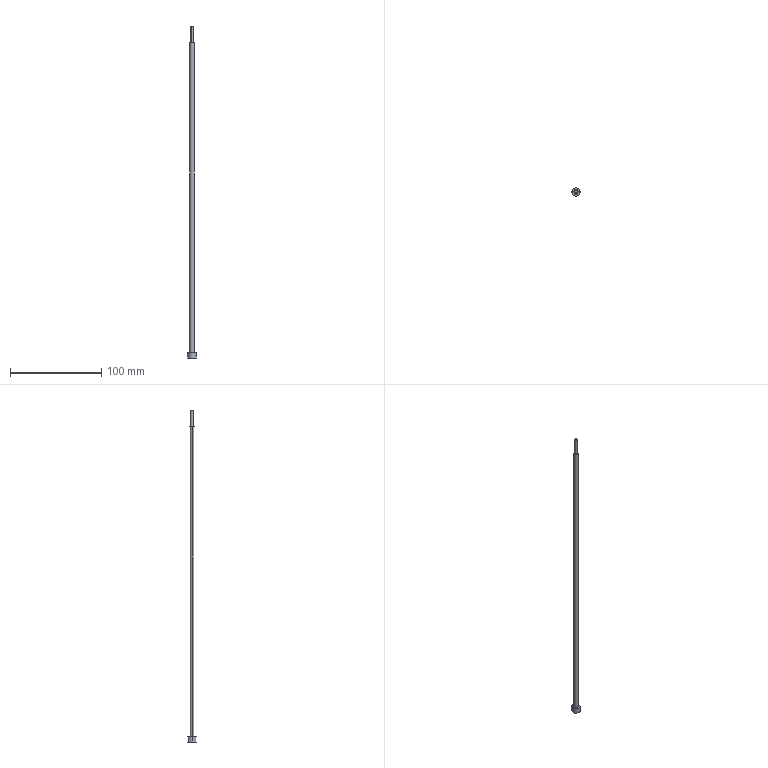Part | Creo | 1 solid | 12 faces | box 9 x 9 x 363.491 mm | volume 5926 mm3 | cylinder 6 | plane 4 | cone 2 | commonest cylinder face diameters 3.214 x2 4.5 x2 9 x2
STEP:
#1=CARTESIAN_POINT('',(-76.601,-142.631,-319.5));
#2=VERTEX_POINT('',#1);
#3=CARTESIAN_POINT('',(-72.101,-142.631,-319.5));
#4=VERTEX_POINT('',#3);
#5=CARTESIAN_POINT('',(-74.351,-142.631,-319.5));
#6=DIRECTION('',(0.,0.,-1.));
#7=DIRECTION('',(-1.,0.,0.));
#8=AXIS2_PLACEMENT_3D('',#5,#6,#7);
#9=CIRCLE('',#8,2.25);
#10=EDGE_CURVE('',#2,#4,#9,.T.);
#11=ORIENTED_EDGE('',*,*,#10,.T.);
#12=CARTESIAN_POINT('',(-72.101,-142.631,19.789));
#13=VERTEX_POINT('',#12);
#14=CARTESIAN_POINT('',(-72.101,-142.631,-319.5));
#15=DIRECTION('',(0.,0.,1.));
#16=VECTOR('',#15,339.289);
#17=LINE('',#14,#16);
#18=EDGE_CURVE('',#4,#13,#17,.T.);
#19=ORIENTED_EDGE('',*,*,#18,.T.);
#20=CARTESIAN_POINT('',(-76.601,-142.631,19.789));
#21=VERTEX_POINT('',#20);
#22=CARTESIAN_POINT('',(-74.351,-142.631,19.789));
#23=DIRECTION('',(0.,0.,1.));
#24=DIRECTION('',(1.,0.,0.));
#25=AXIS2_PLACEMENT_3D('',#22,#23,#24);
#26=CIRCLE('',#25,2.25);
#27=EDGE_CURVE('',#13,#21,#26,.T.);
#28=ORIENTED_EDGE('',*,*,#27,.T.);
#29=CARTESIAN_POINT('',(-76.601,-142.631,-319.5));
#30=DIRECTION('',(0.,0.,1.));
#31=VECTOR('',#30,339.289);
#32=LINE('',#29,#31);
#33=EDGE_CURVE('',#2,#21,#32,.T.);
#34=ORIENTED_EDGE('',*,*,#33,.F.);
#35=EDGE_LOOP('',(#11,#19,#28,#34));
#36=FACE_OUTER_BOUND('',#35,.F.);
#37=CARTESIAN_POINT('',(-74.351,-142.631,-310.5));
#38=DIRECTION('',(0.,0.,1.));
#39=DIRECTION('',(1.,0.,0.));
#40=AXIS2_PLACEMENT_3D('',#37,#38,#39);
#41=CYLINDRICAL_SURFACE('',#40,2.25);
#42=ADVANCED_FACE('',(#36),#41,.T.);
#43=CARTESIAN_POINT('',(-78.851,-142.631,-319.5));
#44=VERTEX_POINT('',#43);
#45=CARTESIAN_POINT('',(-69.851,-142.631,-319.5));
#46=VERTEX_POINT('',#45);
#47=CARTESIAN_POINT('',(-74.351,-142.631,-319.5));
#48=DIRECTION('',(0.,0.,1.));
#49=DIRECTION('',(-1.,0.,0.));
#50=AXIS2_PLACEMENT_3D('',#47,#48,#49);
#51=CIRCLE('',#50,4.5);
#52=EDGE_CURVE('',#44,#46,#51,.T.);
#53=ORIENTED_EDGE('',*,*,#52,.F.);
#54=CARTESIAN_POINT('',(-74.351,-142.631,-319.5));
#55=DIRECTION('',(0.,0.,1.));
#56=DIRECTION('',(1.,0.,0.));
#57=AXIS2_PLACEMENT_3D('',#54,#55,#56);
#58=CIRCLE('',#57,4.5);
#59=EDGE_CURVE('',#46,#44,#58,.T.);
#60=ORIENTED_EDGE('',*,*,#59,.F.);
#61=EDGE_LOOP('',(#53,#60));
#62=FACE_OUTER_BOUND('',#61,.F.);
#63=CARTESIAN_POINT('',(-74.351,-142.631,-319.5));
#64=DIRECTION('',(0.,0.,-1.));
#65=DIRECTION('',(1.,0.,0.));
#66=AXIS2_PLACEMENT_3D('',#63,#64,#65);
#67=CIRCLE('',#66,2.25);
#68=EDGE_CURVE('',#4,#2,#67,.T.);
#69=ORIENTED_EDGE('',*,*,#68,.F.);
#70=ORIENTED_EDGE('',*,*,#10,.F.);
#71=EDGE_LOOP('',(#69,#70));
#72=FACE_BOUND('',#71,.F.);
#73=CARTESIAN_POINT('',(-74.351,-142.631,-319.5));
#74=DIRECTION('',(0.,0.,1.));
#75=DIRECTION('',(1.,0.,0.));
#76=AXIS2_PLACEMENT_3D('',#73,#74,#75);
#77=PLANE('',#76);
#78=ADVANCED_FACE('',(#62,#72),#77,.T.);
#79=ORIENTED_EDGE('',*,*,#68,.T.);
#80=ORIENTED_EDGE('',*,*,#33,.T.);
#81=CARTESIAN_POINT('',(-74.351,-142.631,19.789));
#82=DIRECTION('',(0.,0.,1.));
#83=DIRECTION('',(-1.,0.,0.));
#84=AXIS2_PLACEMENT_3D('',#81,#82,#83);
#85=CIRCLE('',#84,2.25);
#86=EDGE_CURVE('',#21,#13,#85,.T.);
#87=ORIENTED_EDGE('',*,*,#86,.T.);
#88=ORIENTED_EDGE('',*,*,#18,.F.);
#89=EDGE_LOOP('',(#79,#80,#87,#88));
#90=FACE_OUTER_BOUND('',#89,.F.);
#91=CARTESIAN_POINT('',(-74.351,-142.631,-310.5));
#92=DIRECTION('',(0.,0.,1.));
#93=DIRECTION('',(1.,0.,0.));
#94=AXIS2_PLACEMENT_3D('',#91,#92,#93);
#95=CYLINDRICAL_SURFACE('',#94,2.25);
#96=ADVANCED_FACE('',(#90),#95,.T.);
#97=ORIENTED_EDGE('',*,*,#86,.F.);
#98=ORIENTED_EDGE('',*,*,#27,.F.);
#99=EDGE_LOOP('',(#97,#98));
#100=FACE_OUTER_BOUND('',#99,.F.);
#101=CARTESIAN_POINT('',(-74.351,-140.522,19.789));
#102=VERTEX_POINT('',#101);
#103=CARTESIAN_POINT('',(-72.242,-142.631,19.789));
#104=VERTEX_POINT('',#103);
#105=CARTESIAN_POINT('',(-74.351,-142.631,19.789));
#106=DIRECTION('',(0.,0.,-1.));
#107=DIRECTION('',(0.,1.,0.));
#108=AXIS2_PLACEMENT_3D('',#105,#106,#107);
#109=CIRCLE('',#108,2.109);
#110=EDGE_CURVE('',#102,#104,#109,.T.);
#111=ORIENTED_EDGE('',*,*,#110,.F.);
#112=CARTESIAN_POINT('',(-76.461,-142.631,19.789));
#113=VERTEX_POINT('',#112);
#114=CARTESIAN_POINT('',(-74.351,-142.631,19.789));
#115=DIRECTION('',(0.,0.,-1.));
#116=DIRECTION('',(-1.,0.,0.));
#117=AXIS2_PLACEMENT_3D('',#114,#115,#116);
#118=CIRCLE('',#117,2.109);
#119=EDGE_CURVE('',#113,#102,#118,.T.);
#120=ORIENTED_EDGE('',*,*,#119,.F.);
#121=CARTESIAN_POINT('',(-74.351,-142.631,19.789));
#122=DIRECTION('',(0.,0.,-1.));
#123=DIRECTION('',(1.,0.,0.));
#124=AXIS2_PLACEMENT_3D('',#121,#122,#123);
#125=CIRCLE('',#124,2.109);
#126=EDGE_CURVE('',#104,#113,#125,.T.);
#127=ORIENTED_EDGE('',*,*,#126,.F.);
#128=EDGE_LOOP('',(#111,#120,#127));
#129=FACE_BOUND('',#128,.F.);
#130=CARTESIAN_POINT('',(-0.003698,-18.777,19.789));
#131=DIRECTION('',(0.,0.,-1.));
#132=DIRECTION('',(0.,-1.,0.));
#133=AXIS2_PLACEMENT_3D('',#130,#131,#132);
#134=PLANE('',#133);
#135=ADVANCED_FACE('',(#100,#129),#134,.F.);
#136=CARTESIAN_POINT('',(-74.351,-141.024,20.291));
#137=VERTEX_POINT('',#136);
#138=CARTESIAN_POINT('',(-72.744,-142.631,20.291));
#139=VERTEX_POINT('',#138);
#140=CARTESIAN_POINT('',(-74.351,-142.631,20.291));
#141=DIRECTION('',(0.,0.,-1.));
#142=DIRECTION('',(0.,1.,0.));
#143=AXIS2_PLACEMENT_3D('',#140,#141,#142);
#144=CIRCLE('',#143,1.607);
#145=EDGE_CURVE('',#137,#139,#144,.T.);
#146=ORIENTED_EDGE('',*,*,#145,.F.);
#147=CARTESIAN_POINT('',(-75.959,-142.631,20.291));
#148=VERTEX_POINT('',#147);
#149=CARTESIAN_POINT('',(-74.351,-142.631,20.291));
#150=DIRECTION('',(0.,0.,-1.));
#151=DIRECTION('',(-1.,0.,0.));
#152=AXIS2_PLACEMENT_3D('',#149,#150,#151);
#153=CIRCLE('',#152,1.607);
#154=EDGE_CURVE('',#148,#137,#153,.T.);
#155=ORIENTED_EDGE('',*,*,#154,.F.);
#156=CARTESIAN_POINT('',(-75.959,-142.631,20.291));
#157=DIRECTION('',(-0.7071,0.,-0.7072));
#158=VECTOR('',#157,0.7099);
#159=LINE('',#156,#158);
#160=EDGE_CURVE('',#148,#113,#159,.T.);
#161=ORIENTED_EDGE('',*,*,#160,.T.);
#162=ORIENTED_EDGE('',*,*,#119,.T.);
#163=ORIENTED_EDGE('',*,*,#110,.T.);
#164=CARTESIAN_POINT('',(-72.744,-142.631,20.291));
#165=DIRECTION('',(0.7071,0.,-0.7072));
#166=VECTOR('',#165,0.7099);
#167=LINE('',#164,#166);
#168=EDGE_CURVE('',#139,#104,#167,.T.);
#169=ORIENTED_EDGE('',*,*,#168,.F.);
#170=EDGE_LOOP('',(#146,#155,#161,#162,#163,#169));
#171=FACE_OUTER_BOUND('',#170,.F.);
#172=CARTESIAN_POINT('',(-74.351,-142.631,20.04));
#173=DIRECTION('',(0.,0.,-1.));
#174=DIRECTION('',(1.,0.,0.));
#175=AXIS2_PLACEMENT_3D('',#172,#173,#174);
#176=CONICAL_SURFACE('',#175,1.858,44.996);
#177=ADVANCED_FACE('',(#171),#176,.T.);
#178=CARTESIAN_POINT('',(-74.351,-144.239,37.93));
#179=VERTEX_POINT('',#178);
#180=CARTESIAN_POINT('',(-72.744,-142.631,37.868));
#181=VERTEX_POINT('',#180);
#182=CARTESIAN_POINT('',(-74.351,-144.239,37.93));
#183=CARTESIAN_POINT('',(-74.132,-144.239,37.921));
#184=CARTESIAN_POINT('',(-73.729,-144.156,37.906));
#185=CARTESIAN_POINT('',(-73.188,-143.803,37.885));
#186=CARTESIAN_POINT('',(-72.83,-143.263,37.872));
#187=CARTESIAN_POINT('',(-72.744,-142.854,37.868));
#188=B_SPLINE_CURVE_WITH_KNOTS('',3,(#182,#183,#184,#185,#186,#187,#180),.UNSPECIFIED.,.F.,.F.,(4,1,1,1,4),(0.,0.25,0.5,0.75,1.),.UNSPECIFIED.);
#189=EDGE_CURVE('',#179,#181,#188,.T.);
#190=ORIENTED_EDGE('',*,*,#189,.T.);
#191=CARTESIAN_POINT('',(-74.351,-141.024,37.93));
#192=VERTEX_POINT('',#191);
#193=CARTESIAN_POINT('',(-72.744,-142.631,37.868));
#194=CARTESIAN_POINT('',(-72.744,-142.409,37.868));
#195=CARTESIAN_POINT('',(-72.83,-142.,37.872));
#196=CARTESIAN_POINT('',(-73.188,-141.46,37.885));
#197=CARTESIAN_POINT('',(-73.728,-141.107,37.906));
#198=CARTESIAN_POINT('',(-74.132,-141.024,37.921));
#199=CARTESIAN_POINT('',(-74.351,-141.024,37.93));
#200=B_SPLINE_CURVE_WITH_KNOTS('',3,(#193,#194,#195,#196,#197,#198,#199),.UNSPECIFIED.,.F.,.F.,(4,1,1,1,4),(0.,0.25,0.5,0.75,1.),.UNSPECIFIED.);
#201=EDGE_CURVE('',#181,#192,#200,.T.);
#202=ORIENTED_EDGE('',*,*,#201,.T.);
#203=CARTESIAN_POINT('',(-74.351,-141.024,37.93));
#204=DIRECTION('',(-0.000002985,0.000000828,-1.));
#205=VECTOR('',#204,17.639);
#206=LINE('',#203,#205);
#207=EDGE_CURVE('',#192,#137,#206,.T.);
#208=ORIENTED_EDGE('',*,*,#207,.T.);
#209=ORIENTED_EDGE('',*,*,#145,.T.);
#210=CARTESIAN_POINT('',(-74.351,-144.239,20.291));
#211=VERTEX_POINT('',#210);
#212=CARTESIAN_POINT('',(-74.351,-142.631,20.291));
#213=DIRECTION('',(0.,0.,-1.));
#214=DIRECTION('',(1.,0.,0.));
#215=AXIS2_PLACEMENT_3D('',#212,#213,#214);
#216=CIRCLE('',#215,1.607);
#217=EDGE_CURVE('',#139,#211,#216,.T.);
#218=ORIENTED_EDGE('',*,*,#217,.T.);
#219=CARTESIAN_POINT('',(-74.351,-144.239,37.93));
#220=DIRECTION('',(0.,-0.000000828,-1.));
#221=VECTOR('',#220,17.639);
#222=LINE('',#219,#221);
#223=EDGE_CURVE('',#179,#211,#222,.T.);
#224=ORIENTED_EDGE('',*,*,#223,.F.);
#225=EDGE_LOOP('',(#190,#202,#208,#209,#218,#224));
#226=FACE_OUTER_BOUND('',#225,.F.);
#227=CARTESIAN_POINT('',(-74.351,-142.631,19.789));
#228=DIRECTION('',(0.,0.,-1.));
#229=DIRECTION('',(0.,-1.,0.));
#230=AXIS2_PLACEMENT_3D('',#227,#228,#229);
#231=CYLINDRICAL_SURFACE('',#230,1.607);
#232=ADVANCED_FACE('',(#226),#231,.T.);
#233=CARTESIAN_POINT('',(-75.959,-142.631,37.991));
#234=VERTEX_POINT('',#233);
#235=CARTESIAN_POINT('',(-74.351,-141.024,37.93));
#236=CARTESIAN_POINT('',(-74.571,-141.024,37.938));
#237=CARTESIAN_POINT('',(-74.974,-141.107,37.954));
#238=CARTESIAN_POINT('',(-75.514,-141.46,37.974));
#239=CARTESIAN_POINT('',(-75.873,-142.,37.988));
#240=CARTESIAN_POINT('',(-75.959,-142.409,37.991));
#241=CARTESIAN_POINT('',(-75.959,-142.631,37.991));
#242=B_SPLINE_CURVE_WITH_KNOTS('',3,(#235,#236,#237,#238,#239,#240,#241),.UNSPECIFIED.,.F.,.F.,(4,1,1,1,4),(0.,0.25,0.5,0.75,1.),.UNSPECIFIED.);
#243=EDGE_CURVE('',#192,#234,#242,.T.);
#244=ORIENTED_EDGE('',*,*,#243,.F.);
#245=ORIENTED_EDGE('',*,*,#201,.F.);
#246=ORIENTED_EDGE('',*,*,#189,.F.);
#247=CARTESIAN_POINT('',(-75.959,-142.809,37.991));
#248=CARTESIAN_POINT('',(-75.902,-143.142,37.989));
#249=CARTESIAN_POINT('',(-75.668,-143.597,37.98));
#250=CARTESIAN_POINT('',(-75.308,-143.955,37.966));
#251=CARTESIAN_POINT('',(-74.853,-144.185,37.949));
#252=CARTESIAN_POINT('',(-74.525,-144.239,37.936));
#253=CARTESIAN_POINT('',(-74.351,-144.239,37.93));
#254=B_SPLINE_CURVE_WITH_KNOTS('',3,(#233,#247,#248,#249,#250,#251,#252,#253),.UNSPECIFIED.,.F.,.F.,(4,1,1,1,1,4),(0.,0.2,0.4,0.6,0.8,1.),.UNSPECIFIED.);
#255=EDGE_CURVE('',#234,#179,#254,.T.);
#256=ORIENTED_EDGE('',*,*,#255,.F.);
#257=EDGE_LOOP('',(#244,#245,#246,#256));
#258=FACE_OUTER_BOUND('',#257,.F.);
#259=CARTESIAN_POINT('',(-122.791,-167.242,39.779));
#260=DIRECTION('',(-0.03814,0.,-0.9993));
#261=DIRECTION('',(-0.9993,0.,0.03814));
#262=AXIS2_PLACEMENT_3D('',#259,#260,#261);
#263=PLANE('',#262);
#264=ADVANCED_FACE('',(#258),#263,.F.);
#265=ORIENTED_EDGE('',*,*,#255,.T.);
#266=ORIENTED_EDGE('',*,*,#223,.T.);
#267=CARTESIAN_POINT('',(-74.351,-142.631,20.291));
#268=DIRECTION('',(0.,0.,-1.));
#269=DIRECTION('',(0.,-1.,0.));
#270=AXIS2_PLACEMENT_3D('',#267,#268,#269);
#271=CIRCLE('',#270,1.607);
#272=EDGE_CURVE('',#211,#148,#271,.T.);
#273=ORIENTED_EDGE('',*,*,#272,.T.);
#274=ORIENTED_EDGE('',*,*,#154,.T.);
#275=ORIENTED_EDGE('',*,*,#207,.F.);
#276=ORIENTED_EDGE('',*,*,#243,.T.);
#277=EDGE_LOOP('',(#265,#266,#273,#274,#275,#276));
#278=FACE_OUTER_BOUND('',#277,.F.);
#279=CARTESIAN_POINT('',(-74.351,-142.631,19.789));
#280=DIRECTION('',(0.,0.,-1.));
#281=DIRECTION('',(0.,-1.,0.));
#282=AXIS2_PLACEMENT_3D('',#279,#280,#281);
#283=CYLINDRICAL_SURFACE('',#282,1.607);
#284=ADVANCED_FACE('',(#278),#283,.T.);
#285=ORIENTED_EDGE('',*,*,#217,.F.);
#286=ORIENTED_EDGE('',*,*,#168,.T.);
#287=ORIENTED_EDGE('',*,*,#126,.T.);
#288=ORIENTED_EDGE('',*,*,#160,.F.);
#289=ORIENTED_EDGE('',*,*,#272,.F.);
#290=EDGE_LOOP('',(#285,#286,#287,#288,#289));
#291=FACE_OUTER_BOUND('',#290,.F.);
#292=CARTESIAN_POINT('',(-74.351,-142.631,20.04));
#293=DIRECTION('',(0.,0.,-1.));
#294=DIRECTION('',(1.,0.,0.));
#295=AXIS2_PLACEMENT_3D('',#292,#293,#294);
#296=CONICAL_SURFACE('',#295,1.858,44.996);
#297=ADVANCED_FACE('',(#291),#296,.T.);
#298=ORIENTED_EDGE('',*,*,#52,.T.);
#299=CARTESIAN_POINT('',(-69.851,-142.631,-325.5));
#300=VERTEX_POINT('',#299);
#301=CARTESIAN_POINT('',(-69.851,-142.631,-325.5));
#302=DIRECTION('',(0.,0.,1.));
#303=VECTOR('',#302,6.);
#304=LINE('',#301,#303);
#305=EDGE_CURVE('',#300,#46,#304,.T.);
#306=ORIENTED_EDGE('',*,*,#305,.F.);
#307=CARTESIAN_POINT('',(-78.851,-142.631,-325.5));
#308=VERTEX_POINT('',#307);
#309=CARTESIAN_POINT('',(-74.351,-142.631,-325.5));
#310=DIRECTION('',(0.,0.,-1.));
#311=DIRECTION('',(1.,0.,0.));
#312=AXIS2_PLACEMENT_3D('',#309,#310,#311);
#313=CIRCLE('',#312,4.5);
#314=EDGE_CURVE('',#300,#308,#313,.T.);
#315=ORIENTED_EDGE('',*,*,#314,.T.);
#316=CARTESIAN_POINT('',(-78.851,-142.631,-325.5));
#317=DIRECTION('',(0.,0.,1.));
#318=VECTOR('',#317,6.);
#319=LINE('',#316,#318);
#320=EDGE_CURVE('',#308,#44,#319,.T.);
#321=ORIENTED_EDGE('',*,*,#320,.T.);
#322=EDGE_LOOP('',(#298,#306,#315,#321));
#323=FACE_OUTER_BOUND('',#322,.F.);
#324=CARTESIAN_POINT('',(-74.351,-142.631,-325.5));
#325=DIRECTION('',(0.,0.,1.));
#326=DIRECTION('',(1.,0.,0.));
#327=AXIS2_PLACEMENT_3D('',#324,#325,#326);
#328=CYLINDRICAL_SURFACE('',#327,4.5);
#329=ADVANCED_FACE('',(#323),#328,.T.);
#330=ORIENTED_EDGE('',*,*,#59,.T.);
#331=ORIENTED_EDGE('',*,*,#320,.F.);
#332=CARTESIAN_POINT('',(-74.351,-142.631,-325.5));
#333=DIRECTION('',(0.,0.,-1.));
#334=DIRECTION('',(-1.,0.,0.));
#335=AXIS2_PLACEMENT_3D('',#332,#333,#334);
#336=CIRCLE('',#335,4.5);
#337=EDGE_CURVE('',#308,#300,#336,.T.);
#338=ORIENTED_EDGE('',*,*,#337,.T.);
#339=ORIENTED_EDGE('',*,*,#305,.T.);
#340=EDGE_LOOP('',(#330,#331,#338,#339));
#341=FACE_OUTER_BOUND('',#340,.F.);
#342=CARTESIAN_POINT('',(-74.351,-142.631,-325.5));
#343=DIRECTION('',(0.,0.,1.));
#344=DIRECTION('',(1.,0.,0.));
#345=AXIS2_PLACEMENT_3D('',#342,#343,#344);
#346=CYLINDRICAL_SURFACE('',#345,4.5);
#347=ADVANCED_FACE('',(#341),#346,.T.);
#348=ORIENTED_EDGE('',*,*,#314,.F.);
#349=ORIENTED_EDGE('',*,*,#337,.F.);
#350=EDGE_LOOP('',(#348,#349));
#351=FACE_OUTER_BOUND('',#350,.F.);
#352=CARTESIAN_POINT('',(-74.351,-142.631,-325.5));
#353=DIRECTION('',(0.,0.,-1.));
#354=DIRECTION('',(-1.,0.,0.));
#355=AXIS2_PLACEMENT_3D('',#352,#353,#354);
#356=PLANE('',#355);
#357=ADVANCED_FACE('',(#351),#356,.T.);
#358=CLOSED_SHELL('',(#42,#78,#96,#135,#177,#232,#264,#284,#297,#329,#347,#357));
#359=MANIFOLD_SOLID_BREP('',#358);
#360=(LENGTH_UNIT()NAMED_UNIT(*)SI_UNIT(.MILLI.,.METRE.));
#361=UNCERTAINTY_MEASURE_WITH_UNIT(LENGTH_MEASURE(0.03637),#360,'','');
#362=(NAMED_UNIT(*)PLANE_ANGLE_UNIT()SI_UNIT($,.RADIAN.));
#363=PLANE_ANGLE_MEASURE_WITH_UNIT(PLANE_ANGLE_MEASURE(0.01745),#362);
#364=(CONVERSION_BASED_UNIT('DEGREE',#363)NAMED_UNIT(*)PLANE_ANGLE_UNIT());
#365=(NAMED_UNIT(*)SI_UNIT($,.STERADIAN.)SOLID_ANGLE_UNIT());
#366=(GEOMETRIC_REPRESENTATION_CONTEXT(3)GLOBAL_UNCERTAINTY_ASSIGNED_CONTEXT((#361))GLOBAL_UNIT_ASSIGNED_CONTEXT((#360,#364,#365))REPRESENTATION_CONTEXT('',''));
#367=ADVANCED_BREP_SHAPE_REPRESENTATION('',(#359),#366);